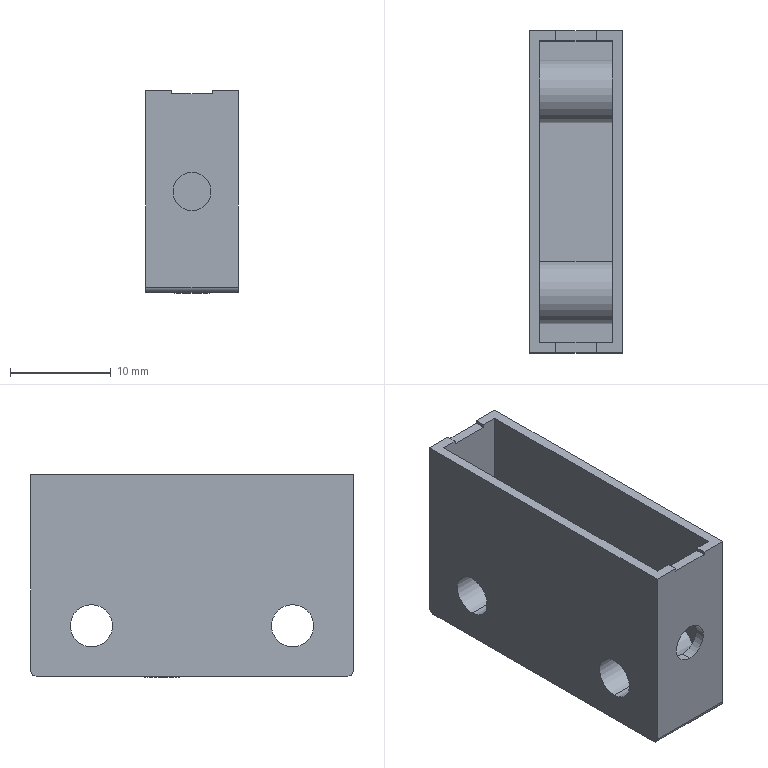Part | SolidWorks | features ICE 8, Fillet 2, Extrusion 1 | 1 solid | 33 faces | box 9.2 x 32 x 20.1 mm | volume 1950 mm3 | plane 19 | cylinder 14 | commonest cylinder face diameters 4.2 x4 6.2 x4 1 x2 3.482 x2 3.8 x2
STEP:
#1=CARTESIAN_POINT('',(-3.6,9.1,-5.));
#2=VERTEX_POINT('',#1);
#3=CARTESIAN_POINT('',(-3.6,2.9,-5.));
#4=VERTEX_POINT('',#3);
#5=CARTESIAN_POINT('',(-3.6,6.,-5.));
#6=DIRECTION('',(1.,0.,0.));
#7=DIRECTION('',(0.,-1.,0.));
#8=AXIS2_PLACEMENT_3D('',#5,#6,#7);
#9=CIRCLE('',#8,3.1);
#10=EDGE_CURVE('',#2,#4,#9,.T.);
#11=ORIENTED_EDGE('',*,*,#10,.T.);
#12=CARTESIAN_POINT('',(3.6,2.9,-5.));
#13=VERTEX_POINT('',#12);
#14=CARTESIAN_POINT('',(-12.368,2.9,-5.));
#15=DIRECTION('',(1.,0.,0.));
#16=VECTOR('',#15,1000.);
#17=LINE('',#14,#16);
#18=EDGE_CURVE('',#4,#13,#17,.T.);
#19=ORIENTED_EDGE('',*,*,#18,.T.);
#20=CARTESIAN_POINT('',(3.6,9.1,-5.));
#21=VERTEX_POINT('',#20);
#22=CARTESIAN_POINT('',(3.6,6.,-5.));
#23=DIRECTION('',(-1.,0.,0.));
#24=DIRECTION('',(0.,1.,0.));
#25=AXIS2_PLACEMENT_3D('',#22,#23,#24);
#26=CIRCLE('',#25,3.1);
#27=EDGE_CURVE('',#13,#21,#26,.T.);
#28=ORIENTED_EDGE('',*,*,#27,.T.);
#29=CARTESIAN_POINT('',(-12.368,9.1,-5.));
#30=DIRECTION('',(1.,0.,0.));
#31=VECTOR('',#30,1000.);
#32=LINE('',#29,#31);
#33=EDGE_CURVE('',#2,#21,#32,.T.);
#34=ORIENTED_EDGE('',*,*,#33,.F.);
#35=EDGE_LOOP('',(#11,#19,#28,#34));
#36=FACE_OUTER_BOUND('',#35,.T.);
#37=CARTESIAN_POINT('',(-12.368,6.,-5.));
#38=DIRECTION('',(1.,0.,0.));
#39=DIRECTION('',(0.,1.,0.));
#40=AXIS2_PLACEMENT_3D('',#37,#38,#39);
#41=CYLINDRICAL_SURFACE('',#40,3.1);
#42=ADVANCED_FACE('',(#36),#41,.T.);
#43=CARTESIAN_POINT('',(-3.6,29.1,-5.));
#44=VERTEX_POINT('',#43);
#45=CARTESIAN_POINT('',(-3.6,22.9,-5.));
#46=VERTEX_POINT('',#45);
#47=CARTESIAN_POINT('',(-3.6,26.,-5.));
#48=DIRECTION('',(1.,0.,0.));
#49=DIRECTION('',(0.,-1.,0.));
#50=AXIS2_PLACEMENT_3D('',#47,#48,#49);
#51=CIRCLE('',#50,3.1);
#52=EDGE_CURVE('',#44,#46,#51,.T.);
#53=ORIENTED_EDGE('',*,*,#52,.T.);
#54=CARTESIAN_POINT('',(3.6,22.9,-5.));
#55=VERTEX_POINT('',#54);
#56=CARTESIAN_POINT('',(-12.368,22.9,-5.));
#57=DIRECTION('',(1.,0.,0.));
#58=VECTOR('',#57,1000.);
#59=LINE('',#56,#58);
#60=EDGE_CURVE('',#46,#55,#59,.T.);
#61=ORIENTED_EDGE('',*,*,#60,.T.);
#62=CARTESIAN_POINT('',(3.6,29.1,-5.));
#63=VERTEX_POINT('',#62);
#64=CARTESIAN_POINT('',(3.6,26.,-5.));
#65=DIRECTION('',(-1.,0.,0.));
#66=DIRECTION('',(0.,1.,0.));
#67=AXIS2_PLACEMENT_3D('',#64,#65,#66);
#68=CIRCLE('',#67,3.1);
#69=EDGE_CURVE('',#55,#63,#68,.T.);
#70=ORIENTED_EDGE('',*,*,#69,.T.);
#71=CARTESIAN_POINT('',(-12.368,29.1,-5.));
#72=DIRECTION('',(1.,0.,0.));
#73=VECTOR('',#72,1000.);
#74=LINE('',#71,#73);
#75=EDGE_CURVE('',#44,#63,#74,.T.);
#76=ORIENTED_EDGE('',*,*,#75,.F.);
#77=EDGE_LOOP('',(#53,#61,#70,#76));
#78=FACE_OUTER_BOUND('',#77,.T.);
#79=CARTESIAN_POINT('',(-12.368,26.,-5.));
#80=DIRECTION('',(1.,0.,0.));
#81=DIRECTION('',(0.,1.,0.));
#82=AXIS2_PLACEMENT_3D('',#79,#80,#81);
#83=CYLINDRICAL_SURFACE('',#82,3.1);
#84=ADVANCED_FACE('',(#78),#83,.T.);
#85=CARTESIAN_POINT('',(0.,1.,1.9));
#86=VERTEX_POINT('',#85);
#87=CARTESIAN_POINT('',(0.,1.,-1.9));
#88=VERTEX_POINT('',#87);
#89=CARTESIAN_POINT('',(0.,1.,0.));
#90=DIRECTION('',(0.,-1.,0.));
#91=DIRECTION('',(0.,0.,-1.));
#92=AXIS2_PLACEMENT_3D('',#89,#90,#91);
#93=CIRCLE('',#92,1.9);
#94=EDGE_CURVE('',#86,#88,#93,.T.);
#95=ORIENTED_EDGE('',*,*,#94,.F.);
#96=CARTESIAN_POINT('',(0.,0.,1.9));
#97=VERTEX_POINT('',#96);
#98=CARTESIAN_POINT('',(0.,17.5,1.9));
#99=DIRECTION('',(0.,-1.,0.));
#100=VECTOR('',#99,1000.);
#101=LINE('',#98,#100);
#102=EDGE_CURVE('',#86,#97,#101,.T.);
#103=ORIENTED_EDGE('',*,*,#102,.T.);
#104=CARTESIAN_POINT('',(0.,0.,-1.9));
#105=VERTEX_POINT('',#104);
#106=CARTESIAN_POINT('',(0.,0.,0.));
#107=DIRECTION('',(0.,-1.,0.));
#108=DIRECTION('',(0.,0.,-1.));
#109=AXIS2_PLACEMENT_3D('',#106,#107,#108);
#110=CIRCLE('',#109,1.9);
#111=EDGE_CURVE('',#97,#105,#110,.T.);
#112=ORIENTED_EDGE('',*,*,#111,.T.);
#113=CARTESIAN_POINT('',(0.,17.5,-1.9));
#114=DIRECTION('',(0.,-1.,0.));
#115=VECTOR('',#114,1000.);
#116=LINE('',#113,#115);
#117=EDGE_CURVE('',#88,#105,#116,.T.);
#118=ORIENTED_EDGE('',*,*,#117,.F.);
#119=EDGE_LOOP('',(#95,#103,#112,#118));
#120=FACE_OUTER_BOUND('',#119,.T.);
#121=CARTESIAN_POINT('',(0.,17.5,0.));
#122=DIRECTION('',(0.,-1.,0.));
#123=DIRECTION('',(0.,0.,-1.));
#124=AXIS2_PLACEMENT_3D('',#121,#122,#123);
#125=CYLINDRICAL_SURFACE('',#124,1.9);
#126=ADVANCED_FACE('',(#120),#125,.F.);
#127=CARTESIAN_POINT('',(-1.741,18.962,-10.1));
#128=VERTEX_POINT('',#127);
#129=CARTESIAN_POINT('',(1.741,18.962,-10.1));
#130=VERTEX_POINT('',#129);
#131=CARTESIAN_POINT('',(0.,18.962,-10.1));
#132=DIRECTION('',(0.,0.,-1.));
#133=DIRECTION('',(-1.,0.,0.));
#134=AXIS2_PLACEMENT_3D('',#131,#132,#133);
#135=CIRCLE('',#134,1.741);
#136=EDGE_CURVE('',#128,#130,#135,.T.);
#137=ORIENTED_EDGE('',*,*,#136,.F.);
#138=CARTESIAN_POINT('',(-1.741,18.962,-10.));
#139=VERTEX_POINT('',#138);
#140=CARTESIAN_POINT('',(-1.741,18.962,-10.1));
#141=DIRECTION('',(0.,0.,1.));
#142=VECTOR('',#141,1000.);
#143=LINE('',#140,#142);
#144=EDGE_CURVE('',#128,#139,#143,.T.);
#145=ORIENTED_EDGE('',*,*,#144,.T.);
#146=CARTESIAN_POINT('',(1.741,18.962,-10.));
#147=VERTEX_POINT('',#146);
#148=CARTESIAN_POINT('',(0.,18.962,-10.));
#149=DIRECTION('',(0.,0.,-1.));
#150=DIRECTION('',(-1.,0.,0.));
#151=AXIS2_PLACEMENT_3D('',#148,#149,#150);
#152=CIRCLE('',#151,1.741);
#153=EDGE_CURVE('',#139,#147,#152,.T.);
#154=ORIENTED_EDGE('',*,*,#153,.T.);
#155=CARTESIAN_POINT('',(1.741,18.962,-10.1));
#156=DIRECTION('',(0.,0.,1.));
#157=VECTOR('',#156,1000.);
#158=LINE('',#155,#157);
#159=EDGE_CURVE('',#130,#147,#158,.T.);
#160=ORIENTED_EDGE('',*,*,#159,.F.);
#161=EDGE_LOOP('',(#137,#145,#154,#160));
#162=FACE_OUTER_BOUND('',#161,.T.);
#163=CARTESIAN_POINT('',(0.,18.962,-10.1));
#164=DIRECTION('',(0.,0.,1.));
#165=DIRECTION('',(1.,0.,0.));
#166=AXIS2_PLACEMENT_3D('',#163,#164,#165);
#167=CYLINDRICAL_SURFACE('',#166,1.741);
#168=ADVANCED_FACE('',(#162),#167,.T.);
#169=CARTESIAN_POINT('',(-4.6,26.,-2.9));
#170=VERTEX_POINT('',#169);
#171=CARTESIAN_POINT('',(-4.6,26.,-7.1));
#172=VERTEX_POINT('',#171);
#173=CARTESIAN_POINT('',(-4.6,26.,-5.));
#174=DIRECTION('',(1.,0.,0.));
#175=DIRECTION('',(0.,0.,-1.));
#176=AXIS2_PLACEMENT_3D('',#173,#174,#175);
#177=CIRCLE('',#176,2.1);
#178=EDGE_CURVE('',#170,#172,#177,.T.);
#179=ORIENTED_EDGE('',*,*,#178,.F.);
#180=CARTESIAN_POINT('',(4.6,26.,-2.9));
#181=VERTEX_POINT('',#180);
#182=CARTESIAN_POINT('',(-4.6,26.,-2.9));
#183=DIRECTION('',(1.,0.,0.));
#184=VECTOR('',#183,1000.);
#185=LINE('',#182,#184);
#186=EDGE_CURVE('',#170,#181,#185,.T.);
#187=ORIENTED_EDGE('',*,*,#186,.T.);
#188=CARTESIAN_POINT('',(4.6,26.,-7.1));
#189=VERTEX_POINT('',#188);
#190=CARTESIAN_POINT('',(4.6,26.,-5.));
#191=DIRECTION('',(1.,0.,0.));
#192=DIRECTION('',(0.,0.,-1.));
#193=AXIS2_PLACEMENT_3D('',#190,#191,#192);
#194=CIRCLE('',#193,2.1);
#195=EDGE_CURVE('',#181,#189,#194,.T.);
#196=ORIENTED_EDGE('',*,*,#195,.T.);
#197=CARTESIAN_POINT('',(-4.6,26.,-7.1));
#198=DIRECTION('',(1.,0.,0.));
#199=VECTOR('',#198,1000.);
#200=LINE('',#197,#199);
#201=EDGE_CURVE('',#172,#189,#200,.T.);
#202=ORIENTED_EDGE('',*,*,#201,.F.);
#203=EDGE_LOOP('',(#179,#187,#196,#202));
#204=FACE_OUTER_BOUND('',#203,.T.);
#205=CARTESIAN_POINT('',(-4.6,26.,-5.));
#206=DIRECTION('',(1.,0.,0.));
#207=DIRECTION('',(0.,0.,-1.));
#208=AXIS2_PLACEMENT_3D('',#205,#206,#207);
#209=CYLINDRICAL_SURFACE('',#208,2.1);
#210=ADVANCED_FACE('',(#204),#209,.F.);
#211=CARTESIAN_POINT('',(-4.6,6.,-2.9));
#212=VERTEX_POINT('',#211);
#213=CARTESIAN_POINT('',(-4.6,6.,-7.1));
#214=VERTEX_POINT('',#213);
#215=CARTESIAN_POINT('',(-4.6,6.,-5.));
#216=DIRECTION('',(1.,0.,0.));
#217=DIRECTION('',(0.,0.,-1.));
#218=AXIS2_PLACEMENT_3D('',#215,#216,#217);
#219=CIRCLE('',#218,2.1);
#220=EDGE_CURVE('',#212,#214,#219,.T.);
#221=ORIENTED_EDGE('',*,*,#220,.F.);
#222=CARTESIAN_POINT('',(4.6,6.,-2.9));
#223=VERTEX_POINT('',#222);
#224=CARTESIAN_POINT('',(-4.6,6.,-2.9));
#225=DIRECTION('',(1.,0.,0.));
#226=VECTOR('',#225,1000.);
#227=LINE('',#224,#226);
#228=EDGE_CURVE('',#212,#223,#227,.T.);
#229=ORIENTED_EDGE('',*,*,#228,.T.);
#230=CARTESIAN_POINT('',(4.6,6.,-7.1));
#231=VERTEX_POINT('',#230);
#232=CARTESIAN_POINT('',(4.6,6.,-5.));
#233=DIRECTION('',(1.,0.,0.));
#234=DIRECTION('',(0.,0.,-1.));
#235=AXIS2_PLACEMENT_3D('',#232,#233,#234);
#236=CIRCLE('',#235,2.1);
#237=EDGE_CURVE('',#223,#231,#236,.T.);
#238=ORIENTED_EDGE('',*,*,#237,.T.);
#239=CARTESIAN_POINT('',(-4.6,6.,-7.1));
#240=DIRECTION('',(1.,0.,0.));
#241=VECTOR('',#240,1000.);
#242=LINE('',#239,#241);
#243=EDGE_CURVE('',#214,#231,#242,.T.);
#244=ORIENTED_EDGE('',*,*,#243,.F.);
#245=EDGE_LOOP('',(#221,#229,#238,#244));
#246=FACE_OUTER_BOUND('',#245,.T.);
#247=CARTESIAN_POINT('',(-4.6,6.,-5.));
#248=DIRECTION('',(1.,0.,0.));
#249=DIRECTION('',(0.,0.,-1.));
#250=AXIS2_PLACEMENT_3D('',#247,#248,#249);
#251=CYLINDRICAL_SURFACE('',#250,2.1);
#252=ADVANCED_FACE('',(#246),#251,.F.);
#253=ORIENTED_EDGE('',*,*,#52,.F.);
#254=CARTESIAN_POINT('',(-3.6,26.,-5.));
#255=DIRECTION('',(1.,0.,0.));
#256=DIRECTION('',(0.,-1.,0.));
#257=AXIS2_PLACEMENT_3D('',#254,#255,#256);
#258=CIRCLE('',#257,3.1);
#259=EDGE_CURVE('',#46,#44,#258,.T.);
#260=ORIENTED_EDGE('',*,*,#259,.F.);
#261=EDGE_LOOP('',(#253,#260));
#262=FACE_BOUND('',#261,.T.);
#263=CARTESIAN_POINT('',(-3.6,31.,10.));
#264=VERTEX_POINT('',#263);
#265=CARTESIAN_POINT('',(-3.6,1.,10.));
#266=VERTEX_POINT('',#265);
#267=CARTESIAN_POINT('',(-3.6,31.,10.));
#268=DIRECTION('',(0.,-1.,0.));
#269=VECTOR('',#268,1000.);
#270=LINE('',#267,#269);
#271=EDGE_CURVE('',#264,#266,#270,.T.);
#272=ORIENTED_EDGE('',*,*,#271,.T.);
#273=CARTESIAN_POINT('',(-3.6,1.,-9.));
#274=VERTEX_POINT('',#273);
#275=CARTESIAN_POINT('',(-3.6,1.,-9.));
#276=DIRECTION('',(0.,0.,1.));
#277=VECTOR('',#276,1000.);
#278=LINE('',#275,#277);
#279=EDGE_CURVE('',#274,#266,#278,.T.);
#280=ORIENTED_EDGE('',*,*,#279,.F.);
#281=CARTESIAN_POINT('',(-3.6,31.,-9.));
#282=VERTEX_POINT('',#281);
#283=CARTESIAN_POINT('',(-3.6,31.,-9.));
#284=DIRECTION('',(0.,-1.,0.));
#285=VECTOR('',#284,1000.);
#286=LINE('',#283,#285);
#287=EDGE_CURVE('',#282,#274,#286,.T.);
#288=ORIENTED_EDGE('',*,*,#287,.F.);
#289=CARTESIAN_POINT('',(-3.6,31.,-9.));
#290=DIRECTION('',(0.,0.,1.));
#291=VECTOR('',#290,1000.);
#292=LINE('',#289,#291);
#293=EDGE_CURVE('',#282,#264,#292,.T.);
#294=ORIENTED_EDGE('',*,*,#293,.T.);
#295=EDGE_LOOP('',(#272,#280,#288,#294));
#296=FACE_OUTER_BOUND('',#295,.T.);
#297=ORIENTED_EDGE('',*,*,#10,.F.);
#298=CARTESIAN_POINT('',(-3.6,6.,-5.));
#299=DIRECTION('',(1.,0.,0.));
#300=DIRECTION('',(0.,-1.,0.));
#301=AXIS2_PLACEMENT_3D('',#298,#299,#300);
#302=CIRCLE('',#301,3.1);
#303=EDGE_CURVE('',#4,#2,#302,.T.);
#304=ORIENTED_EDGE('',*,*,#303,.F.);
#305=EDGE_LOOP('',(#297,#304));
#306=FACE_BOUND('',#305,.T.);
#307=CARTESIAN_POINT('',(-3.6,31.,-9.));
#308=DIRECTION('',(-1.,0.,0.));
#309=DIRECTION('',(0.,-1.,0.));
#310=AXIS2_PLACEMENT_3D('',#307,#308,#309);
#311=PLANE('',#310);
#312=ADVANCED_FACE('',(#262,#296,#306),#311,.F.);
#313=CARTESIAN_POINT('',(3.6,26.,-5.));
#314=DIRECTION('',(-1.,0.,0.));
#315=DIRECTION('',(0.,1.,0.));
#316=AXIS2_PLACEMENT_3D('',#313,#314,#315);
#317=CIRCLE('',#316,3.1);
#318=EDGE_CURVE('',#63,#55,#317,.T.);
#319=ORIENTED_EDGE('',*,*,#318,.F.);
#320=ORIENTED_EDGE('',*,*,#69,.F.);
#321=EDGE_LOOP('',(#319,#320));
#322=FACE_BOUND('',#321,.T.);
#323=CARTESIAN_POINT('',(3.6,1.,10.));
#324=VERTEX_POINT('',#323);
#325=CARTESIAN_POINT('',(3.6,31.,10.));
#326=VERTEX_POINT('',#325);
#327=CARTESIAN_POINT('',(3.6,31.,10.));
#328=DIRECTION('',(0.,1.,0.));
#329=VECTOR('',#328,1000.);
#330=LINE('',#327,#329);
#331=EDGE_CURVE('',#324,#326,#330,.T.);
#332=ORIENTED_EDGE('',*,*,#331,.T.);
#333=CARTESIAN_POINT('',(3.6,31.,-9.));
#334=VERTEX_POINT('',#333);
#335=CARTESIAN_POINT('',(3.6,31.,-9.));
#336=DIRECTION('',(0.,0.,1.));
#337=VECTOR('',#336,1000.);
#338=LINE('',#335,#337);
#339=EDGE_CURVE('',#334,#326,#338,.T.);
#340=ORIENTED_EDGE('',*,*,#339,.F.);
#341=CARTESIAN_POINT('',(3.6,1.,-9.));
#342=VERTEX_POINT('',#341);
#343=CARTESIAN_POINT('',(3.6,31.,-9.));
#344=DIRECTION('',(0.,1.,0.));
#345=VECTOR('',#344,1000.);
#346=LINE('',#343,#345);
#347=EDGE_CURVE('',#342,#334,#346,.T.);
#348=ORIENTED_EDGE('',*,*,#347,.F.);
#349=CARTESIAN_POINT('',(3.6,1.,-9.));
#350=DIRECTION('',(0.,0.,1.));
#351=VECTOR('',#350,1000.);
#352=LINE('',#349,#351);
#353=EDGE_CURVE('',#342,#324,#352,.T.);
#354=ORIENTED_EDGE('',*,*,#353,.T.);
#355=EDGE_LOOP('',(#332,#340,#348,#354));
#356=FACE_OUTER_BOUND('',#355,.T.);
#357=CARTESIAN_POINT('',(3.6,6.,-5.));
#358=DIRECTION('',(-1.,0.,0.));
#359=DIRECTION('',(0.,1.,0.));
#360=AXIS2_PLACEMENT_3D('',#357,#358,#359);
#361=CIRCLE('',#360,3.1);
#362=EDGE_CURVE('',#21,#13,#361,.T.);
#363=ORIENTED_EDGE('',*,*,#362,.F.);
#364=ORIENTED_EDGE('',*,*,#27,.F.);
#365=EDGE_LOOP('',(#363,#364));
#366=FACE_BOUND('',#365,.T.);
#367=CARTESIAN_POINT('',(3.6,31.,-9.));
#368=DIRECTION('',(1.,0.,0.));
#369=DIRECTION('',(0.,1.,0.));
#370=AXIS2_PLACEMENT_3D('',#367,#368,#369);
#371=PLANE('',#370);
#372=ADVANCED_FACE('',(#322,#356,#366),#371,.F.);
#373=CARTESIAN_POINT('',(-2.,32.,10.));
#374=VERTEX_POINT('',#373);
#375=CARTESIAN_POINT('',(-2.,31.,10.));
#376=VERTEX_POINT('',#375);
#377=CARTESIAN_POINT('',(-2.,32.,10.));
#378=DIRECTION('',(0.,-1.,0.));
#379=VECTOR('',#378,1000.);
#380=LINE('',#377,#379);
#381=EDGE_CURVE('',#374,#376,#380,.T.);
#382=ORIENTED_EDGE('',*,*,#381,.T.);
#383=CARTESIAN_POINT('',(-2.,31.,9.7));
#384=VERTEX_POINT('',#383);
#385=CARTESIAN_POINT('',(-2.,31.,10.));
#386=DIRECTION('',(0.,0.,-1.));
#387=VECTOR('',#386,1000.);
#388=LINE('',#385,#387);
#389=EDGE_CURVE('',#376,#384,#388,.T.);
#390=ORIENTED_EDGE('',*,*,#389,.T.);
#391=CARTESIAN_POINT('',(-2.,32.,9.7));
#392=VERTEX_POINT('',#391);
#393=CARTESIAN_POINT('',(-2.,32.,9.7));
#394=DIRECTION('',(0.,-1.,0.));
#395=VECTOR('',#394,1000.);
#396=LINE('',#393,#395);
#397=EDGE_CURVE('',#392,#384,#396,.T.);
#398=ORIENTED_EDGE('',*,*,#397,.F.);
#399=CARTESIAN_POINT('',(-2.,32.,10.));
#400=DIRECTION('',(0.,0.,-1.));
#401=VECTOR('',#400,1000.);
#402=LINE('',#399,#401);
#403=EDGE_CURVE('',#374,#392,#402,.T.);
#404=ORIENTED_EDGE('',*,*,#403,.F.);
#405=EDGE_LOOP('',(#382,#390,#398,#404));
#406=FACE_OUTER_BOUND('',#405,.T.);
#407=CARTESIAN_POINT('',(-2.,32.,10.));
#408=DIRECTION('',(-1.,0.,0.));
#409=DIRECTION('',(0.,0.,1.));
#410=AXIS2_PLACEMENT_3D('',#407,#408,#409);
#411=PLANE('',#410);
#412=ADVANCED_FACE('',(#406),#411,.F.);
#413=ORIENTED_EDGE('',*,*,#397,.T.);
#414=CARTESIAN_POINT('',(2.,31.,9.7));
#415=VERTEX_POINT('',#414);
#416=CARTESIAN_POINT('',(-2.,31.,9.7));
#417=DIRECTION('',(1.,0.,0.));
#418=VECTOR('',#417,1000.);
#419=LINE('',#416,#418);
#420=EDGE_CURVE('',#384,#415,#419,.T.);
#421=ORIENTED_EDGE('',*,*,#420,.T.);
#422=CARTESIAN_POINT('',(2.,32.,9.7));
#423=VERTEX_POINT('',#422);
#424=CARTESIAN_POINT('',(2.,32.,9.7));
#425=DIRECTION('',(0.,-1.,0.));
#426=VECTOR('',#425,1000.);
#427=LINE('',#424,#426);
#428=EDGE_CURVE('',#423,#415,#427,.T.);
#429=ORIENTED_EDGE('',*,*,#428,.F.);
#430=CARTESIAN_POINT('',(-2.,32.,9.7));
#431=DIRECTION('',(1.,0.,0.));
#432=VECTOR('',#431,1000.);
#433=LINE('',#430,#432);
#434=EDGE_CURVE('',#392,#423,#433,.T.);
#435=ORIENTED_EDGE('',*,*,#434,.F.);
#436=EDGE_LOOP('',(#413,#421,#429,#435));
#437=FACE_OUTER_BOUND('',#436,.T.);
#438=CARTESIAN_POINT('',(-2.,32.,9.7));
#439=DIRECTION('',(0.,0.,-1.));
#440=DIRECTION('',(-1.,0.,0.));
#441=AXIS2_PLACEMENT_3D('',#438,#439,#440);
#442=PLANE('',#441);
#443=ADVANCED_FACE('',(#437),#442,.F.);
#444=ORIENTED_EDGE('',*,*,#428,.T.);
#445=CARTESIAN_POINT('',(2.,31.,10.));
#446=VERTEX_POINT('',#445);
#447=CARTESIAN_POINT('',(2.,31.,10.));
#448=DIRECTION('',(0.,0.,1.));
#449=VECTOR('',#448,1000.);
#450=LINE('',#447,#449);
#451=EDGE_CURVE('',#415,#446,#450,.T.);
#452=ORIENTED_EDGE('',*,*,#451,.T.);
#453=CARTESIAN_POINT('',(2.,32.,10.));
#454=VERTEX_POINT('',#453);
#455=CARTESIAN_POINT('',(2.,32.,10.));
#456=DIRECTION('',(0.,-1.,0.));
#457=VECTOR('',#456,1000.);
#458=LINE('',#455,#457);
#459=EDGE_CURVE('',#454,#446,#458,.T.);
#460=ORIENTED_EDGE('',*,*,#459,.F.);
#461=CARTESIAN_POINT('',(2.,32.,10.));
#462=DIRECTION('',(0.,0.,1.));
#463=VECTOR('',#462,1000.);
#464=LINE('',#461,#463);
#465=EDGE_CURVE('',#423,#454,#464,.T.);
#466=ORIENTED_EDGE('',*,*,#465,.F.);
#467=EDGE_LOOP('',(#444,#452,#460,#466));
#468=FACE_OUTER_BOUND('',#467,.T.);
#469=CARTESIAN_POINT('',(2.,32.,10.));
#470=DIRECTION('',(1.,0.,0.));
#471=DIRECTION('',(0.,0.,-1.));
#472=AXIS2_PLACEMENT_3D('',#469,#470,#471);
#473=PLANE('',#472);
#474=ADVANCED_FACE('',(#468),#473,.F.);
#475=CARTESIAN_POINT('',(4.6,26.,-5.));
#476=DIRECTION('',(1.,0.,0.));
#477=DIRECTION('',(0.,0.,-1.));
#478=AXIS2_PLACEMENT_3D('',#475,#476,#477);
#479=CIRCLE('',#478,2.1);
#480=EDGE_CURVE('',#189,#181,#479,.T.);
#481=ORIENTED_EDGE('',*,*,#480,.F.);
#482=ORIENTED_EDGE('',*,*,#195,.F.);
#483=EDGE_LOOP('',(#481,#482));
#484=FACE_BOUND('',#483,.T.);
#485=CARTESIAN_POINT('',(4.6,6.,-5.));
#486=DIRECTION('',(1.,0.,0.));
#487=DIRECTION('',(0.,0.,-1.));
#488=AXIS2_PLACEMENT_3D('',#485,#486,#487);
#489=CIRCLE('',#488,2.1);
#490=EDGE_CURVE('',#231,#223,#489,.T.);
#491=ORIENTED_EDGE('',*,*,#490,.F.);
#492=ORIENTED_EDGE('',*,*,#237,.F.);
#493=EDGE_LOOP('',(#491,#492));
#494=FACE_BOUND('',#493,.T.);
#495=CARTESIAN_POINT('',(4.6,0.,10.));
#496=VERTEX_POINT('',#495);
#497=CARTESIAN_POINT('',(4.6,0.,-9.5));
#498=VERTEX_POINT('',#497);
#499=CARTESIAN_POINT('',(4.6,0.,10.));
#500=DIRECTION('',(0.,0.,-1.));
#501=VECTOR('',#500,1000.);
#502=LINE('',#499,#501);
#503=EDGE_CURVE('',#496,#498,#502,.T.);
#504=ORIENTED_EDGE('',*,*,#503,.T.);
#505=CARTESIAN_POINT('',(4.6,0.5,-10.));
#506=VERTEX_POINT('',#505);
#507=CARTESIAN_POINT('',(4.6,0.5,-9.5));
#508=DIRECTION('',(1.,0.,0.));
#509=DIRECTION('',(0.,0.,1.));
#510=AXIS2_PLACEMENT_3D('',#507,#508,#509);
#511=CIRCLE('',#510,0.5);
#512=EDGE_CURVE('',#498,#506,#511,.T.);
#513=ORIENTED_EDGE('',*,*,#512,.T.);
#514=CARTESIAN_POINT('',(4.6,31.5,-10.));
#515=VERTEX_POINT('',#514);
#516=CARTESIAN_POINT('',(4.6,32.,-10.));
#517=DIRECTION('',(0.,-1.,0.));
#518=VECTOR('',#517,1000.);
#519=LINE('',#516,#518);
#520=EDGE_CURVE('',#515,#506,#519,.T.);
#521=ORIENTED_EDGE('',*,*,#520,.F.);
#522=CARTESIAN_POINT('',(4.6,32.,-9.5));
#523=VERTEX_POINT('',#522);
#524=CARTESIAN_POINT('',(4.6,31.5,-9.5));
#525=DIRECTION('',(1.,0.,0.));
#526=DIRECTION('',(0.,0.,1.));
#527=AXIS2_PLACEMENT_3D('',#524,#525,#526);
#528=CIRCLE('',#527,0.5);
#529=EDGE_CURVE('',#515,#523,#528,.T.);
#530=ORIENTED_EDGE('',*,*,#529,.T.);
#531=CARTESIAN_POINT('',(4.6,32.,10.));
#532=VERTEX_POINT('',#531);
#533=CARTESIAN_POINT('',(4.6,32.,10.));
#534=DIRECTION('',(0.,0.,-1.));
#535=VECTOR('',#534,1000.);
#536=LINE('',#533,#535);
#537=EDGE_CURVE('',#532,#523,#536,.T.);
#538=ORIENTED_EDGE('',*,*,#537,.F.);
#539=CARTESIAN_POINT('',(4.6,32.,10.));
#540=DIRECTION('',(0.,-1.,0.));
#541=VECTOR('',#540,1000.);
#542=LINE('',#539,#541);
#543=EDGE_CURVE('',#532,#496,#542,.T.);
#544=ORIENTED_EDGE('',*,*,#543,.T.);
#545=EDGE_LOOP('',(#504,#513,#521,#530,#538,#544));
#546=FACE_OUTER_BOUND('',#545,.T.);
#547=CARTESIAN_POINT('',(4.6,32.,10.));
#548=DIRECTION('',(-1.,0.,0.));
#549=DIRECTION('',(0.,0.,1.));
#550=AXIS2_PLACEMENT_3D('',#547,#548,#549);
#551=PLANE('',#550);
#552=ADVANCED_FACE('',(#484,#494,#546),#551,.F.);
#553=CARTESIAN_POINT('',(0.,18.962,-10.));
#554=DIRECTION('',(0.,0.,-1.));
#555=DIRECTION('',(-1.,0.,0.));
#556=AXIS2_PLACEMENT_3D('',#553,#554,#555);
#557=CIRCLE('',#556,1.741);
#558=EDGE_CURVE('',#147,#139,#557,.T.);
#559=ORIENTED_EDGE('',*,*,#558,.F.);
#560=ORIENTED_EDGE('',*,*,#153,.F.);
#561=EDGE_LOOP('',(#559,#560));
#562=FACE_BOUND('',#561,.T.);
#563=ORIENTED_EDGE('',*,*,#520,.T.);
#564=CARTESIAN_POINT('',(-4.6,0.5,-10.));
#565=VERTEX_POINT('',#564);
#566=CARTESIAN_POINT('',(-4.6,0.5,-10.));
#567=DIRECTION('',(-1.,0.,0.));
#568=VECTOR('',#567,1000.);
#569=LINE('',#566,#568);
#570=EDGE_CURVE('',#506,#565,#569,.T.);
#571=ORIENTED_EDGE('',*,*,#570,.T.);
#572=CARTESIAN_POINT('',(-4.6,31.5,-10.));
#573=VERTEX_POINT('',#572);
#574=CARTESIAN_POINT('',(-4.6,32.,-10.));
#575=DIRECTION('',(0.,-1.,0.));
#576=VECTOR('',#575,1000.);
#577=LINE('',#574,#576);
#578=EDGE_CURVE('',#573,#565,#577,.T.);
#579=ORIENTED_EDGE('',*,*,#578,.F.);
#580=CARTESIAN_POINT('',(-4.6,31.5,-10.));
#581=DIRECTION('',(1.,0.,0.));
#582=VECTOR('',#581,1000.);
#583=LINE('',#580,#582);
#584=EDGE_CURVE('',#573,#515,#583,.T.);
#585=ORIENTED_EDGE('',*,*,#584,.T.);
#586=EDGE_LOOP('',(#563,#571,#579,#585));
#587=FACE_OUTER_BOUND('',#586,.T.);
#588=CARTESIAN_POINT('',(-4.6,32.,-10.));
#589=DIRECTION('',(0.,0.,1.));
#590=DIRECTION('',(1.,0.,0.));
#591=AXIS2_PLACEMENT_3D('',#588,#589,#590);
#592=PLANE('',#591);
#593=ADVANCED_FACE('',(#562,#587),#592,.F.);
#594=CARTESIAN_POINT('',(-4.6,26.,-5.));
#595=DIRECTION('',(1.,0.,0.));
#596=DIRECTION('',(0.,0.,-1.));
#597=AXIS2_PLACEMENT_3D('',#594,#595,#596);
#598=CIRCLE('',#597,2.1);
#599=EDGE_CURVE('',#172,#170,#598,.T.);
#600=ORIENTED_EDGE('',*,*,#599,.T.);
#601=ORIENTED_EDGE('',*,*,#178,.T.);
#602=EDGE_LOOP('',(#600,#601));
#603=FACE_BOUND('',#602,.T.);
#604=CARTESIAN_POINT('',(-4.6,6.,-5.));
#605=DIRECTION('',(1.,0.,0.));
#606=DIRECTION('',(0.,0.,-1.));
#607=AXIS2_PLACEMENT_3D('',#604,#605,#606);
#608=CIRCLE('',#607,2.1);
#609=EDGE_CURVE('',#214,#212,#608,.T.);
#610=ORIENTED_EDGE('',*,*,#609,.T.);
#611=ORIENTED_EDGE('',*,*,#220,.T.);
#612=EDGE_LOOP('',(#610,#611));
#613=FACE_BOUND('',#612,.T.);
#614=ORIENTED_EDGE('',*,*,#578,.T.);
#615=CARTESIAN_POINT('',(-4.6,0.,-9.5));
#616=VERTEX_POINT('',#615);
#617=CARTESIAN_POINT('',(-4.6,0.5,-9.5));
#618=DIRECTION('',(-1.,0.,0.));
#619=DIRECTION('',(0.,0.,-1.));
#620=AXIS2_PLACEMENT_3D('',#617,#618,#619);
#621=CIRCLE('',#620,0.5);
#622=EDGE_CURVE('',#565,#616,#621,.T.);
#623=ORIENTED_EDGE('',*,*,#622,.T.);
#624=CARTESIAN_POINT('',(-4.6,0.,10.));
#625=VERTEX_POINT('',#624);
#626=CARTESIAN_POINT('',(-4.6,0.,10.));
#627=DIRECTION('',(0.,0.,1.));
#628=VECTOR('',#627,1000.);
#629=LINE('',#626,#628);
#630=EDGE_CURVE('',#616,#625,#629,.T.);
#631=ORIENTED_EDGE('',*,*,#630,.T.);
#632=CARTESIAN_POINT('',(-4.6,32.,10.));
#633=VERTEX_POINT('',#632);
#634=CARTESIAN_POINT('',(-4.6,32.,10.));
#635=DIRECTION('',(0.,-1.,0.));
#636=VECTOR('',#635,1000.);
#637=LINE('',#634,#636);
#638=EDGE_CURVE('',#633,#625,#637,.T.);
#639=ORIENTED_EDGE('',*,*,#638,.F.);
#640=CARTESIAN_POINT('',(-4.6,32.,-9.5));
#641=VERTEX_POINT('',#640);
#642=CARTESIAN_POINT('',(-4.6,32.,10.));
#643=DIRECTION('',(0.,0.,1.));
#644=VECTOR('',#643,1000.);
#645=LINE('',#642,#644);
#646=EDGE_CURVE('',#641,#633,#645,.T.);
#647=ORIENTED_EDGE('',*,*,#646,.F.);
#648=CARTESIAN_POINT('',(-4.6,31.5,-9.5));
#649=DIRECTION('',(-1.,0.,0.));
#650=DIRECTION('',(0.,0.,-1.));
#651=AXIS2_PLACEMENT_3D('',#648,#649,#650);
#652=CIRCLE('',#651,0.5);
#653=EDGE_CURVE('',#641,#573,#652,.T.);
#654=ORIENTED_EDGE('',*,*,#653,.T.);
#655=EDGE_LOOP('',(#614,#623,#631,#639,#647,#654));
#656=FACE_OUTER_BOUND('',#655,.T.);
#657=CARTESIAN_POINT('',(-4.6,32.,10.));
#658=DIRECTION('',(1.,0.,0.));
#659=DIRECTION('',(0.,0.,-1.));
#660=AXIS2_PLACEMENT_3D('',#657,#658,#659);
#661=PLANE('',#660);
#662=ADVANCED_FACE('',(#603,#613,#656),#661,.F.);
#663=ORIENTED_EDGE('',*,*,#271,.F.);
#664=CARTESIAN_POINT('',(-3.6,31.,10.));
#665=DIRECTION('',(-1.,0.,0.));
#666=VECTOR('',#665,1000.);
#667=LINE('',#664,#666);
#668=EDGE_CURVE('',#376,#264,#667,.T.);
#669=ORIENTED_EDGE('',*,*,#668,.F.);
#670=ORIENTED_EDGE('',*,*,#381,.F.);
#671=CARTESIAN_POINT('',(-4.6,32.,10.));
#672=DIRECTION('',(1.,0.,0.));
#673=VECTOR('',#672,1000.);
#674=LINE('',#671,#673);
#675=EDGE_CURVE('',#633,#374,#674,.T.);
#676=ORIENTED_EDGE('',*,*,#675,.F.);
#677=ORIENTED_EDGE('',*,*,#638,.T.);
#678=CARTESIAN_POINT('',(-2.,0.,10.));
#679=VERTEX_POINT('',#678);
#680=CARTESIAN_POINT('',(-4.6,0.,10.));
#681=DIRECTION('',(1.,0.,0.));
#682=VECTOR('',#681,1000.);
#683=LINE('',#680,#682);
#684=EDGE_CURVE('',#625,#679,#683,.T.);
#685=ORIENTED_EDGE('',*,*,#684,.T.);
#686=CARTESIAN_POINT('',(-2.,1.,10.));
#687=VERTEX_POINT('',#686);
#688=CARTESIAN_POINT('',(-2.,32.,10.));
#689=DIRECTION('',(0.,-1.,0.));
#690=VECTOR('',#689,1000.);
#691=LINE('',#688,#690);
#692=EDGE_CURVE('',#687,#679,#691,.T.);
#693=ORIENTED_EDGE('',*,*,#692,.F.);
#694=CARTESIAN_POINT('',(-3.6,1.,10.));
#695=DIRECTION('',(1.,0.,0.));
#696=VECTOR('',#695,1000.);
#697=LINE('',#694,#696);
#698=EDGE_CURVE('',#266,#687,#697,.T.);
#699=ORIENTED_EDGE('',*,*,#698,.F.);
#700=EDGE_LOOP('',(#663,#669,#670,#676,#677,#685,#693,#699));
#701=FACE_OUTER_BOUND('',#700,.T.);
#702=CARTESIAN_POINT('',(-4.6,32.,10.));
#703=DIRECTION('',(0.,0.,-1.));
#704=DIRECTION('',(-1.,0.,0.));
#705=AXIS2_PLACEMENT_3D('',#702,#703,#704);
#706=PLANE('',#705);
#707=ADVANCED_FACE('',(#701),#706,.F.);
#708=CARTESIAN_POINT('',(-2.,1.,9.7));
#709=VERTEX_POINT('',#708);
#710=CARTESIAN_POINT('',(-2.,0.,9.7));
#711=VERTEX_POINT('',#710);
#712=CARTESIAN_POINT('',(-2.,32.,9.7));
#713=DIRECTION('',(0.,-1.,0.));
#714=VECTOR('',#713,1000.);
#715=LINE('',#712,#714);
#716=EDGE_CURVE('',#709,#711,#715,.T.);
#717=ORIENTED_EDGE('',*,*,#716,.F.);
#718=CARTESIAN_POINT('',(-2.,1.,10.));
#719=DIRECTION('',(0.,0.,1.));
#720=VECTOR('',#719,1000.);
#721=LINE('',#718,#720);
#722=EDGE_CURVE('',#709,#687,#721,.T.);
#723=ORIENTED_EDGE('',*,*,#722,.T.);
#724=ORIENTED_EDGE('',*,*,#692,.T.);
#725=CARTESIAN_POINT('',(-2.,0.,10.));
#726=DIRECTION('',(0.,0.,-1.));
#727=VECTOR('',#726,1000.);
#728=LINE('',#725,#727);
#729=EDGE_CURVE('',#679,#711,#728,.T.);
#730=ORIENTED_EDGE('',*,*,#729,.T.);
#731=EDGE_LOOP('',(#717,#723,#724,#730));
#732=FACE_OUTER_BOUND('',#731,.T.);
#733=CARTESIAN_POINT('',(-2.,32.,10.));
#734=DIRECTION('',(-1.,0.,0.));
#735=DIRECTION('',(0.,0.,1.));
#736=AXIS2_PLACEMENT_3D('',#733,#734,#735);
#737=PLANE('',#736);
#738=ADVANCED_FACE('',(#732),#737,.F.);
#739=CARTESIAN_POINT('',(2.,1.,9.7));
#740=VERTEX_POINT('',#739);
#741=CARTESIAN_POINT('',(2.,0.,9.7));
#742=VERTEX_POINT('',#741);
#743=CARTESIAN_POINT('',(2.,32.,9.7));
#744=DIRECTION('',(0.,-1.,0.));
#745=VECTOR('',#744,1000.);
#746=LINE('',#743,#745);
#747=EDGE_CURVE('',#740,#742,#746,.T.);
#748=ORIENTED_EDGE('',*,*,#747,.F.);
#749=CARTESIAN_POINT('',(-2.,1.,9.7));
#750=DIRECTION('',(-1.,0.,0.));
#751=VECTOR('',#750,1000.);
#752=LINE('',#749,#751);
#753=EDGE_CURVE('',#740,#709,#752,.T.);
#754=ORIENTED_EDGE('',*,*,#753,.T.);
#755=ORIENTED_EDGE('',*,*,#716,.T.);
#756=CARTESIAN_POINT('',(-2.,0.,9.7));
#757=DIRECTION('',(1.,0.,0.));
#758=VECTOR('',#757,1000.);
#759=LINE('',#756,#758);
#760=EDGE_CURVE('',#711,#742,#759,.T.);
#761=ORIENTED_EDGE('',*,*,#760,.T.);
#762=EDGE_LOOP('',(#748,#754,#755,#761));
#763=FACE_OUTER_BOUND('',#762,.T.);
#764=CARTESIAN_POINT('',(-2.,32.,9.7));
#765=DIRECTION('',(0.,0.,-1.));
#766=DIRECTION('',(-1.,0.,0.));
#767=AXIS2_PLACEMENT_3D('',#764,#765,#766);
#768=PLANE('',#767);
#769=ADVANCED_FACE('',(#763),#768,.F.);
#770=CARTESIAN_POINT('',(2.,1.,10.));
#771=VERTEX_POINT('',#770);
#772=CARTESIAN_POINT('',(2.,0.,10.));
#773=VERTEX_POINT('',#772);
#774=CARTESIAN_POINT('',(2.,32.,10.));
#775=DIRECTION('',(0.,-1.,0.));
#776=VECTOR('',#775,1000.);
#777=LINE('',#774,#776);
#778=EDGE_CURVE('',#771,#773,#777,.T.);
#779=ORIENTED_EDGE('',*,*,#778,.F.);
#780=CARTESIAN_POINT('',(2.,1.,10.));
#781=DIRECTION('',(0.,0.,-1.));
#782=VECTOR('',#781,1000.);
#783=LINE('',#780,#782);
#784=EDGE_CURVE('',#771,#740,#783,.T.);
#785=ORIENTED_EDGE('',*,*,#784,.T.);
#786=ORIENTED_EDGE('',*,*,#747,.T.);
#787=CARTESIAN_POINT('',(2.,0.,10.));
#788=DIRECTION('',(0.,0.,1.));
#789=VECTOR('',#788,1000.);
#790=LINE('',#787,#789);
#791=EDGE_CURVE('',#742,#773,#790,.T.);
#792=ORIENTED_EDGE('',*,*,#791,.T.);
#793=EDGE_LOOP('',(#779,#785,#786,#792));
#794=FACE_OUTER_BOUND('',#793,.T.);
#795=CARTESIAN_POINT('',(2.,32.,10.));
#796=DIRECTION('',(1.,0.,0.));
#797=DIRECTION('',(0.,0.,-1.));
#798=AXIS2_PLACEMENT_3D('',#795,#796,#797);
#799=PLANE('',#798);
#800=ADVANCED_FACE('',(#794),#799,.F.);
#801=ORIENTED_EDGE('',*,*,#459,.T.);
#802=CARTESIAN_POINT('',(-3.6,31.,10.));
#803=DIRECTION('',(-1.,0.,0.));
#804=VECTOR('',#803,1000.);
#805=LINE('',#802,#804);
#806=EDGE_CURVE('',#326,#446,#805,.T.);
#807=ORIENTED_EDGE('',*,*,#806,.F.);
#808=ORIENTED_EDGE('',*,*,#331,.F.);
#809=CARTESIAN_POINT('',(2.,1.,10.));
#810=DIRECTION('',(-1.,0.,0.));
#811=VECTOR('',#810,1000.);
#812=LINE('',#809,#811);
#813=EDGE_CURVE('',#324,#771,#812,.T.);
#814=ORIENTED_EDGE('',*,*,#813,.T.);
#815=ORIENTED_EDGE('',*,*,#778,.T.);
#816=CARTESIAN_POINT('',(2.,0.,10.));
#817=DIRECTION('',(1.,0.,0.));
#818=VECTOR('',#817,1000.);
#819=LINE('',#816,#818);
#820=EDGE_CURVE('',#773,#496,#819,.T.);
#821=ORIENTED_EDGE('',*,*,#820,.T.);
#822=ORIENTED_EDGE('',*,*,#543,.F.);
#823=CARTESIAN_POINT('',(2.,32.,10.));
#824=DIRECTION('',(1.,0.,0.));
#825=VECTOR('',#824,1000.);
#826=LINE('',#823,#825);
#827=EDGE_CURVE('',#454,#532,#826,.T.);
#828=ORIENTED_EDGE('',*,*,#827,.F.);
#829=EDGE_LOOP('',(#801,#807,#808,#814,#815,#821,#822,#828));
#830=FACE_OUTER_BOUND('',#829,.T.);
#831=CARTESIAN_POINT('',(2.,32.,10.));
#832=DIRECTION('',(0.,0.,-1.));
#833=DIRECTION('',(-1.,0.,0.));
#834=AXIS2_PLACEMENT_3D('',#831,#832,#833);
#835=PLANE('',#834);
#836=ADVANCED_FACE('',(#830),#835,.F.);
#837=ORIENTED_EDGE('',*,*,#537,.T.);
#838=CARTESIAN_POINT('',(0.,32.,-9.5));
#839=DIRECTION('',(-1.,0.,0.));
#840=VECTOR('',#839,1000.);
#841=LINE('',#838,#840);
#842=EDGE_CURVE('',#523,#641,#841,.T.);
#843=ORIENTED_EDGE('',*,*,#842,.T.);
#844=ORIENTED_EDGE('',*,*,#646,.T.);
#845=ORIENTED_EDGE('',*,*,#675,.T.);
#846=ORIENTED_EDGE('',*,*,#403,.T.);
#847=ORIENTED_EDGE('',*,*,#434,.T.);
#848=ORIENTED_EDGE('',*,*,#465,.T.);
#849=ORIENTED_EDGE('',*,*,#827,.T.);
#850=EDGE_LOOP('',(#837,#843,#844,#845,#846,#847,#848,#849));
#851=FACE_OUTER_BOUND('',#850,.T.);
#852=CARTESIAN_POINT('',(0.,32.,0.));
#853=DIRECTION('',(0.,-1.,0.));
#854=DIRECTION('',(0.,0.,-1.));
#855=AXIS2_PLACEMENT_3D('',#852,#853,#854);
#856=PLANE('',#855);
#857=ADVANCED_FACE('',(#851),#856,.F.);
#858=CARTESIAN_POINT('',(0.,0.,0.));
#859=DIRECTION('',(0.,-1.,0.));
#860=DIRECTION('',(0.,0.,-1.));
#861=AXIS2_PLACEMENT_3D('',#858,#859,#860);
#862=CIRCLE('',#861,1.9);
#863=EDGE_CURVE('',#105,#97,#862,.T.);
#864=ORIENTED_EDGE('',*,*,#863,.F.);
#865=ORIENTED_EDGE('',*,*,#111,.F.);
#866=EDGE_LOOP('',(#864,#865));
#867=FACE_BOUND('',#866,.T.);
#868=CARTESIAN_POINT('',(4.6,0.,-9.5));
#869=DIRECTION('',(1.,0.,0.));
#870=VECTOR('',#869,1000.);
#871=LINE('',#868,#870);
#872=EDGE_CURVE('',#616,#498,#871,.T.);
#873=ORIENTED_EDGE('',*,*,#872,.T.);
#874=ORIENTED_EDGE('',*,*,#503,.F.);
#875=ORIENTED_EDGE('',*,*,#820,.F.);
#876=ORIENTED_EDGE('',*,*,#791,.F.);
#877=ORIENTED_EDGE('',*,*,#760,.F.);
#878=ORIENTED_EDGE('',*,*,#729,.F.);
#879=ORIENTED_EDGE('',*,*,#684,.F.);
#880=ORIENTED_EDGE('',*,*,#630,.F.);
#881=EDGE_LOOP('',(#873,#874,#875,#876,#877,#878,#879,#880));
#882=FACE_OUTER_BOUND('',#881,.T.);
#883=CARTESIAN_POINT('',(0.,0.,0.));
#884=DIRECTION('',(0.,-1.,0.));
#885=DIRECTION('',(0.,0.,-1.));
#886=AXIS2_PLACEMENT_3D('',#883,#884,#885);
#887=PLANE('',#886);
#888=ADVANCED_FACE('',(#867,#882),#887,.T.);
#889=ORIENTED_EDGE('',*,*,#228,.F.);
#890=ORIENTED_EDGE('',*,*,#609,.F.);
#891=ORIENTED_EDGE('',*,*,#243,.T.);
#892=ORIENTED_EDGE('',*,*,#490,.T.);
#893=EDGE_LOOP('',(#889,#890,#891,#892));
#894=FACE_OUTER_BOUND('',#893,.T.);
#895=CARTESIAN_POINT('',(-4.6,6.,-5.));
#896=DIRECTION('',(1.,0.,0.));
#897=DIRECTION('',(0.,0.,-1.));
#898=AXIS2_PLACEMENT_3D('',#895,#896,#897);
#899=CYLINDRICAL_SURFACE('',#898,2.1);
#900=ADVANCED_FACE('',(#894),#899,.F.);
#901=ORIENTED_EDGE('',*,*,#186,.F.);
#902=ORIENTED_EDGE('',*,*,#599,.F.);
#903=ORIENTED_EDGE('',*,*,#201,.T.);
#904=ORIENTED_EDGE('',*,*,#480,.T.);
#905=EDGE_LOOP('',(#901,#902,#903,#904));
#906=FACE_OUTER_BOUND('',#905,.T.);
#907=CARTESIAN_POINT('',(-4.6,26.,-5.));
#908=DIRECTION('',(1.,0.,0.));
#909=DIRECTION('',(0.,0.,-1.));
#910=AXIS2_PLACEMENT_3D('',#907,#908,#909);
#911=CYLINDRICAL_SURFACE('',#910,2.1);
#912=ADVANCED_FACE('',(#906),#911,.F.);
#913=ORIENTED_EDGE('',*,*,#144,.F.);
#914=CARTESIAN_POINT('',(0.,18.962,-10.1));
#915=DIRECTION('',(0.,0.,-1.));
#916=DIRECTION('',(-1.,0.,0.));
#917=AXIS2_PLACEMENT_3D('',#914,#915,#916);
#918=CIRCLE('',#917,1.741);
#919=EDGE_CURVE('',#130,#128,#918,.T.);
#920=ORIENTED_EDGE('',*,*,#919,.F.);
#921=ORIENTED_EDGE('',*,*,#159,.T.);
#922=ORIENTED_EDGE('',*,*,#558,.T.);
#923=EDGE_LOOP('',(#913,#920,#921,#922));
#924=FACE_OUTER_BOUND('',#923,.T.);
#925=CARTESIAN_POINT('',(0.,18.962,-10.1));
#926=DIRECTION('',(0.,0.,1.));
#927=DIRECTION('',(1.,0.,0.));
#928=AXIS2_PLACEMENT_3D('',#925,#926,#927);
#929=CYLINDRICAL_SURFACE('',#928,1.741);
#930=ADVANCED_FACE('',(#924),#929,.T.);
#931=ORIENTED_EDGE('',*,*,#919,.T.);
#932=ORIENTED_EDGE('',*,*,#136,.T.);
#933=EDGE_LOOP('',(#931,#932));
#934=FACE_OUTER_BOUND('',#933,.T.);
#935=CARTESIAN_POINT('',(0.,18.962,-10.1));
#936=DIRECTION('',(0.,0.,-1.));
#937=DIRECTION('',(-1.,0.,0.));
#938=AXIS2_PLACEMENT_3D('',#935,#936,#937);
#939=PLANE('',#938);
#940=ADVANCED_FACE('',(#934),#939,.T.);
#941=ORIENTED_EDGE('',*,*,#512,.F.);
#942=ORIENTED_EDGE('',*,*,#872,.F.);
#943=ORIENTED_EDGE('',*,*,#622,.F.);
#944=ORIENTED_EDGE('',*,*,#570,.F.);
#945=EDGE_LOOP('',(#941,#942,#943,#944));
#946=FACE_OUTER_BOUND('',#945,.T.);
#947=CARTESIAN_POINT('',(-4.6,0.5,-9.5));
#948=DIRECTION('',(1.,0.,0.));
#949=DIRECTION('',(0.,0.,-1.));
#950=AXIS2_PLACEMENT_3D('',#947,#948,#949);
#951=CYLINDRICAL_SURFACE('',#950,0.5);
#952=ADVANCED_FACE('',(#946),#951,.T.);
#953=ORIENTED_EDGE('',*,*,#529,.F.);
#954=ORIENTED_EDGE('',*,*,#584,.F.);
#955=ORIENTED_EDGE('',*,*,#653,.F.);
#956=ORIENTED_EDGE('',*,*,#842,.F.);
#957=EDGE_LOOP('',(#953,#954,#955,#956));
#958=FACE_OUTER_BOUND('',#957,.T.);
#959=CARTESIAN_POINT('',(0.,31.5,-9.5));
#960=DIRECTION('',(-1.,0.,0.));
#961=DIRECTION('',(0.,0.,1.));
#962=AXIS2_PLACEMENT_3D('',#959,#960,#961);
#963=CYLINDRICAL_SURFACE('',#962,0.5);
#964=ADVANCED_FACE('',(#958),#963,.T.);
#965=ORIENTED_EDGE('',*,*,#668,.T.);
#966=ORIENTED_EDGE('',*,*,#293,.F.);
#967=CARTESIAN_POINT('',(-3.6,31.,-9.));
#968=DIRECTION('',(-1.,0.,0.));
#969=VECTOR('',#968,1000.);
#970=LINE('',#967,#969);
#971=EDGE_CURVE('',#334,#282,#970,.T.);
#972=ORIENTED_EDGE('',*,*,#971,.F.);
#973=ORIENTED_EDGE('',*,*,#339,.T.);
#974=ORIENTED_EDGE('',*,*,#806,.T.);
#975=ORIENTED_EDGE('',*,*,#451,.F.);
#976=ORIENTED_EDGE('',*,*,#420,.F.);
#977=ORIENTED_EDGE('',*,*,#389,.F.);
#978=EDGE_LOOP('',(#965,#966,#972,#973,#974,#975,#976,#977));
#979=FACE_OUTER_BOUND('',#978,.T.);
#980=CARTESIAN_POINT('',(-3.6,31.,-9.));
#981=DIRECTION('',(0.,1.,0.));
#982=DIRECTION('',(0.,0.,1.));
#983=AXIS2_PLACEMENT_3D('',#980,#981,#982);
#984=PLANE('',#983);
#985=ADVANCED_FACE('',(#979),#984,.F.);
#986=CARTESIAN_POINT('',(0.,1.,0.));
#987=DIRECTION('',(0.,-1.,0.));
#988=DIRECTION('',(0.,0.,-1.));
#989=AXIS2_PLACEMENT_3D('',#986,#987,#988);
#990=CIRCLE('',#989,1.9);
#991=EDGE_CURVE('',#88,#86,#990,.T.);
#992=ORIENTED_EDGE('',*,*,#991,.T.);
#993=ORIENTED_EDGE('',*,*,#94,.T.);
#994=EDGE_LOOP('',(#992,#993));
#995=FACE_BOUND('',#994,.T.);
#996=ORIENTED_EDGE('',*,*,#753,.F.);
#997=ORIENTED_EDGE('',*,*,#784,.F.);
#998=ORIENTED_EDGE('',*,*,#813,.F.);
#999=ORIENTED_EDGE('',*,*,#353,.F.);
#1000=CARTESIAN_POINT('',(-3.6,1.,-9.));
#1001=DIRECTION('',(1.,0.,0.));
#1002=VECTOR('',#1001,1000.);
#1003=LINE('',#1000,#1002);
#1004=EDGE_CURVE('',#274,#342,#1003,.T.);
#1005=ORIENTED_EDGE('',*,*,#1004,.F.);
#1006=ORIENTED_EDGE('',*,*,#279,.T.);
#1007=ORIENTED_EDGE('',*,*,#698,.T.);
#1008=ORIENTED_EDGE('',*,*,#722,.F.);
#1009=EDGE_LOOP('',(#996,#997,#998,#999,#1005,#1006,#1007,#1008));
#1010=FACE_OUTER_BOUND('',#1009,.T.);
#1011=CARTESIAN_POINT('',(-3.6,1.,-9.));
#1012=DIRECTION('',(0.,-1.,0.));
#1013=DIRECTION('',(0.,0.,-1.));
#1014=AXIS2_PLACEMENT_3D('',#1011,#1012,#1013);
#1015=PLANE('',#1014);
#1016=ADVANCED_FACE('',(#995,#1010),#1015,.F.);
#1017=ORIENTED_EDGE('',*,*,#287,.T.);
#1018=ORIENTED_EDGE('',*,*,#1004,.T.);
#1019=ORIENTED_EDGE('',*,*,#347,.T.);
#1020=ORIENTED_EDGE('',*,*,#971,.T.);
#1021=EDGE_LOOP('',(#1017,#1018,#1019,#1020));
#1022=FACE_OUTER_BOUND('',#1021,.T.);
#1023=CARTESIAN_POINT('',(0.,0.,-9.));
#1024=DIRECTION('',(0.,0.,1.));
#1025=DIRECTION('',(1.,0.,0.));
#1026=AXIS2_PLACEMENT_3D('',#1023,#1024,#1025);
#1027=PLANE('',#1026);
#1028=ADVANCED_FACE('',(#1022),#1027,.T.);
#1029=ORIENTED_EDGE('',*,*,#102,.F.);
#1030=ORIENTED_EDGE('',*,*,#991,.F.);
#1031=ORIENTED_EDGE('',*,*,#117,.T.);
#1032=ORIENTED_EDGE('',*,*,#863,.T.);
#1033=EDGE_LOOP('',(#1029,#1030,#1031,#1032));
#1034=FACE_OUTER_BOUND('',#1033,.T.);
#1035=CARTESIAN_POINT('',(0.,17.5,0.));
#1036=DIRECTION('',(0.,-1.,0.));
#1037=DIRECTION('',(0.,0.,-1.));
#1038=AXIS2_PLACEMENT_3D('',#1035,#1036,#1037);
#1039=CYLINDRICAL_SURFACE('',#1038,1.9);
#1040=ADVANCED_FACE('',(#1034),#1039,.F.);
#1041=ORIENTED_EDGE('',*,*,#60,.F.);
#1042=ORIENTED_EDGE('',*,*,#259,.T.);
#1043=ORIENTED_EDGE('',*,*,#75,.T.);
#1044=ORIENTED_EDGE('',*,*,#318,.T.);
#1045=EDGE_LOOP('',(#1041,#1042,#1043,#1044));
#1046=FACE_OUTER_BOUND('',#1045,.T.);
#1047=CARTESIAN_POINT('',(-12.368,26.,-5.));
#1048=DIRECTION('',(1.,0.,0.));
#1049=DIRECTION('',(0.,1.,0.));
#1050=AXIS2_PLACEMENT_3D('',#1047,#1048,#1049);
#1051=CYLINDRICAL_SURFACE('',#1050,3.1);
#1052=ADVANCED_FACE('',(#1046),#1051,.T.);
#1053=ORIENTED_EDGE('',*,*,#18,.F.);
#1054=ORIENTED_EDGE('',*,*,#303,.T.);
#1055=ORIENTED_EDGE('',*,*,#33,.T.);
#1056=ORIENTED_EDGE('',*,*,#362,.T.);
#1057=EDGE_LOOP('',(#1053,#1054,#1055,#1056));
#1058=FACE_OUTER_BOUND('',#1057,.T.);
#1059=CARTESIAN_POINT('',(-12.368,6.,-5.));
#1060=DIRECTION('',(1.,0.,0.));
#1061=DIRECTION('',(0.,1.,0.));
#1062=AXIS2_PLACEMENT_3D('',#1059,#1060,#1061);
#1063=CYLINDRICAL_SURFACE('',#1062,3.1);
#1064=ADVANCED_FACE('',(#1058),#1063,.T.);
#1065=CLOSED_SHELL('',(#42,#84,#126,#168,#210,#252,#312,#372,#412,#443,#474,#552,#593,#662,#707,#738,#769,#800,#836,#857,#888,#900,#912,#930,#940,#952,#964,#985,#1016,#1028,#1040,#1052,#1064));
#1066=MANIFOLD_SOLID_BREP('',#1065);
#1067=CARTESIAN_POINT('',(0.,0.,0.));
#1068=DIRECTION('',(0.,0.,1.));
#1069=DIRECTION('',(1.,0.,0.));
#1070=AXIS2_PLACEMENT_3D('',#1067,#1068,#1069);
#1071=(LENGTH_UNIT()NAMED_UNIT(*)SI_UNIT(.MILLI.,.METRE.));
#1072=UNCERTAINTY_MEASURE_WITH_UNIT(LENGTH_MEASURE(0.00001),#1071,'','');
#1073=(NAMED_UNIT(*)PLANE_ANGLE_UNIT()SI_UNIT($,.RADIAN.));
#1074=(NAMED_UNIT(*)SI_UNIT($,.STERADIAN.)SOLID_ANGLE_UNIT());
#1075=(GEOMETRIC_REPRESENTATION_CONTEXT(3)GLOBAL_UNCERTAINTY_ASSIGNED_CONTEXT((#1072))GLOBAL_UNIT_ASSIGNED_CONTEXT((#1071,#1073,#1074))REPRESENTATION_CONTEXT('',''));
#1076=ADVANCED_BREP_SHAPE_REPRESENTATION('',(#1066,#1070),#1075);